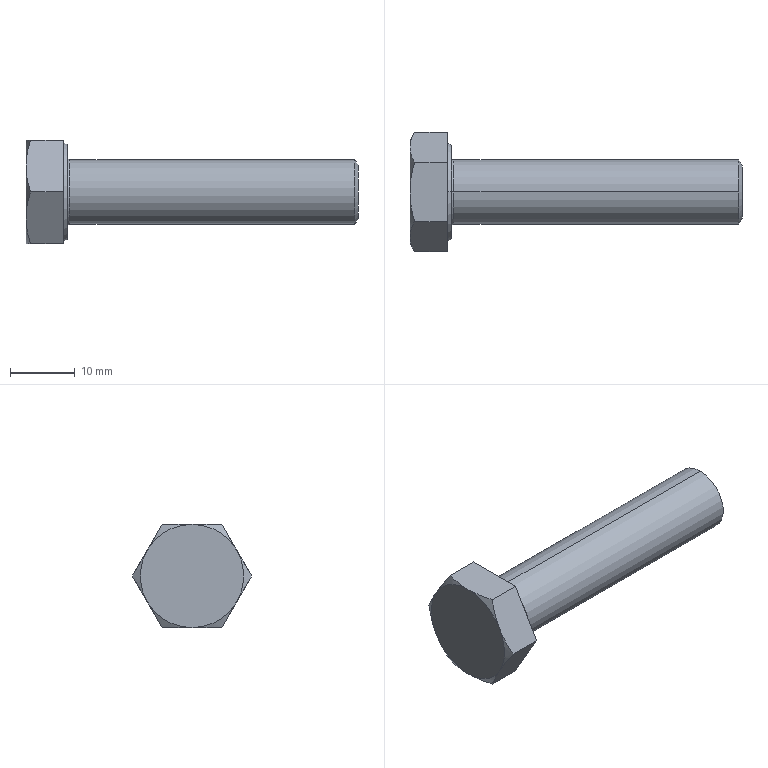Part | SolidWorks | features RevCut 3, Extrusion 1, Fillet 1, LPattern 1, Revolution 1 | 1 solid | 24 faces | box 51.4 x 18.475 x 16 mm | volume 4916 mm3 | cone 10 | plane 10 | torus 2 | cylinder 2 | commonest cylinder face diameters 10 x2
STEP:
#1=CARTESIAN_POINT('',(51.4,0.,4.134));
#2=VERTEX_POINT('',#1);
#3=CARTESIAN_POINT('',(51.4,0.,-4.134));
#4=VERTEX_POINT('',#3);
#5=CARTESIAN_POINT('',(51.4,0.,0.));
#6=DIRECTION('',(-1.,0.,0.));
#7=DIRECTION('',(0.,0.,1.));
#8=AXIS2_PLACEMENT_3D('',#5,#6,#7);
#9=CIRCLE('',#8,4.134);
#10=EDGE_CURVE('',#2,#4,#9,.T.);
#11=ORIENTED_EDGE('',*,*,#10,.T.);
#12=CARTESIAN_POINT('',(50.9,0.,-5.));
#13=VERTEX_POINT('',#12);
#14=CARTESIAN_POINT('',(50.9,0.,-5.));
#15=DIRECTION('',(-0.5,0.,-0.866));
#16=VECTOR('',#15,1000.);
#17=LINE('',#14,#16);
#18=EDGE_CURVE('',#4,#13,#17,.T.);
#19=ORIENTED_EDGE('',*,*,#18,.T.);
#20=CARTESIAN_POINT('',(50.9,0.,5.));
#21=VERTEX_POINT('',#20);
#22=CARTESIAN_POINT('',(50.9,0.,0.));
#23=DIRECTION('',(-1.,0.,0.));
#24=DIRECTION('',(0.,0.,1.));
#25=AXIS2_PLACEMENT_3D('',#22,#23,#24);
#26=CIRCLE('',#25,5.);
#27=EDGE_CURVE('',#21,#13,#26,.T.);
#28=ORIENTED_EDGE('',*,*,#27,.F.);
#29=CARTESIAN_POINT('',(50.9,0.,5.));
#30=DIRECTION('',(-0.5,0.,0.866));
#31=VECTOR('',#30,1000.);
#32=LINE('',#29,#31);
#33=EDGE_CURVE('',#2,#21,#32,.T.);
#34=ORIENTED_EDGE('',*,*,#33,.F.);
#35=EDGE_LOOP('',(#11,#19,#28,#34));
#36=FACE_OUTER_BOUND('',#35,.T.);
#37=CARTESIAN_POINT('',(50.9,0.,0.));
#38=DIRECTION('',(-1.,0.,0.));
#39=DIRECTION('',(0.,0.,1.));
#40=AXIS2_PLACEMENT_3D('',#37,#38,#39);
#41=CONICAL_SURFACE('',#40,5.,1.047);
#42=ADVANCED_FACE('',(#36),#41,.T.);
#43=CARTESIAN_POINT('',(6.8,0.,5.));
#44=VERTEX_POINT('',#43);
#45=CARTESIAN_POINT('',(6.8,0.,-5.));
#46=VERTEX_POINT('',#45);
#47=CARTESIAN_POINT('',(6.8,0.,0.));
#48=DIRECTION('',(1.,0.,0.));
#49=DIRECTION('',(0.,0.,-1.));
#50=AXIS2_PLACEMENT_3D('',#47,#48,#49);
#51=CIRCLE('',#50,5.);
#52=EDGE_CURVE('',#44,#46,#51,.T.);
#53=ORIENTED_EDGE('',*,*,#52,.F.);
#54=CARTESIAN_POINT('',(6.4,0.,5.4));
#55=VERTEX_POINT('',#54);
#56=CARTESIAN_POINT('',(6.8,0.,5.4));
#57=DIRECTION('',(0.,1.,0.));
#58=DIRECTION('',(-1.,0.,0.));
#59=AXIS2_PLACEMENT_3D('',#56,#57,#58);
#60=CIRCLE('',#59,0.4);
#61=EDGE_CURVE('',#44,#55,#60,.T.);
#62=ORIENTED_EDGE('',*,*,#61,.T.);
#63=CARTESIAN_POINT('',(6.4,0.,-5.4));
#64=VERTEX_POINT('',#63);
#65=CARTESIAN_POINT('',(6.4,0.,0.));
#66=DIRECTION('',(-1.,0.,0.));
#67=DIRECTION('',(0.,0.,-1.));
#68=AXIS2_PLACEMENT_3D('',#65,#66,#67);
#69=CIRCLE('',#68,5.4);
#70=EDGE_CURVE('',#64,#55,#69,.T.);
#71=ORIENTED_EDGE('',*,*,#70,.F.);
#72=CARTESIAN_POINT('',(6.8,0.,-5.4));
#73=DIRECTION('',(0.,-1.,0.));
#74=DIRECTION('',(1.,0.,0.));
#75=AXIS2_PLACEMENT_3D('',#72,#73,#74);
#76=CIRCLE('',#75,0.4);
#77=EDGE_CURVE('',#46,#64,#76,.T.);
#78=ORIENTED_EDGE('',*,*,#77,.F.);
#79=EDGE_LOOP('',(#53,#62,#71,#78));
#80=FACE_OUTER_BOUND('',#79,.T.);
#81=CARTESIAN_POINT('',(6.8,0.,0.));
#82=DIRECTION('',(1.,0.,0.));
#83=DIRECTION('',(0.,0.,-1.));
#84=AXIS2_PLACEMENT_3D('',#81,#82,#83);
#85=TOROIDAL_SURFACE('',#84,5.4,0.4);
#86=ADVANCED_FACE('',(#80),#85,.F.);
#87=CARTESIAN_POINT('',(6.4,0.,7.315));
#88=VERTEX_POINT('',#87);
#89=CARTESIAN_POINT('',(6.4,0.,-7.315));
#90=VERTEX_POINT('',#89);
#91=CARTESIAN_POINT('',(6.4,0.,0.));
#92=DIRECTION('',(-1.,0.,0.));
#93=DIRECTION('',(0.,0.,1.));
#94=AXIS2_PLACEMENT_3D('',#91,#92,#93);
#95=CIRCLE('',#94,7.315);
#96=EDGE_CURVE('',#88,#90,#95,.T.);
#97=ORIENTED_EDGE('',*,*,#96,.T.);
#98=CARTESIAN_POINT('',(5.8,0.,-7.661));
#99=VERTEX_POINT('',#98);
#100=CARTESIAN_POINT('',(5.8,0.,-7.661));
#101=DIRECTION('',(-0.866,0.,-0.5));
#102=VECTOR('',#101,1000.);
#103=LINE('',#100,#102);
#104=EDGE_CURVE('',#90,#99,#103,.T.);
#105=ORIENTED_EDGE('',*,*,#104,.T.);
#106=CARTESIAN_POINT('',(5.8,0.,7.661));
#107=VERTEX_POINT('',#106);
#108=CARTESIAN_POINT('',(5.8,0.,0.));
#109=DIRECTION('',(-1.,0.,0.));
#110=DIRECTION('',(0.,0.,1.));
#111=AXIS2_PLACEMENT_3D('',#108,#109,#110);
#112=CIRCLE('',#111,7.661);
#113=EDGE_CURVE('',#107,#99,#112,.T.);
#114=ORIENTED_EDGE('',*,*,#113,.F.);
#115=CARTESIAN_POINT('',(5.8,0.,7.661));
#116=DIRECTION('',(-0.866,0.,0.5));
#117=VECTOR('',#116,1000.);
#118=LINE('',#115,#117);
#119=EDGE_CURVE('',#88,#107,#118,.T.);
#120=ORIENTED_EDGE('',*,*,#119,.F.);
#121=EDGE_LOOP('',(#97,#105,#114,#120));
#122=FACE_OUTER_BOUND('',#121,.T.);
#123=CARTESIAN_POINT('',(5.8,0.,0.));
#124=DIRECTION('',(-1.,0.,0.));
#125=DIRECTION('',(0.,0.,1.));
#126=AXIS2_PLACEMENT_3D('',#123,#124,#125);
#127=CONICAL_SURFACE('',#126,7.661,0.5236);
#128=ADVANCED_FACE('',(#122),#127,.T.);
#129=ORIENTED_EDGE('',*,*,#27,.T.);
#130=CARTESIAN_POINT('',(0.,0.,-5.));
#131=DIRECTION('',(-1.,0.,0.));
#132=VECTOR('',#131,1000.);
#133=LINE('',#130,#132);
#134=EDGE_CURVE('',#13,#46,#133,.T.);
#135=ORIENTED_EDGE('',*,*,#134,.T.);
#136=CARTESIAN_POINT('',(6.8,0.,0.));
#137=DIRECTION('',(1.,0.,0.));
#138=DIRECTION('',(0.,0.,-1.));
#139=AXIS2_PLACEMENT_3D('',#136,#137,#138);
#140=CIRCLE('',#139,5.);
#141=EDGE_CURVE('',#46,#44,#140,.T.);
#142=ORIENTED_EDGE('',*,*,#141,.T.);
#143=CARTESIAN_POINT('',(0.,0.,5.));
#144=DIRECTION('',(-1.,0.,0.));
#145=VECTOR('',#144,1000.);
#146=LINE('',#143,#145);
#147=EDGE_CURVE('',#21,#44,#146,.T.);
#148=ORIENTED_EDGE('',*,*,#147,.F.);
#149=EDGE_LOOP('',(#129,#135,#142,#148));
#150=FACE_OUTER_BOUND('',#149,.T.);
#151=CARTESIAN_POINT('',(0.,0.,0.));
#152=DIRECTION('',(-1.,0.,0.));
#153=DIRECTION('',(0.,0.,1.));
#154=AXIS2_PLACEMENT_3D('',#151,#152,#153);
#155=CYLINDRICAL_SURFACE('',#154,5.);
#156=ADVANCED_FACE('',(#150),#155,.T.);
#157=ORIENTED_EDGE('',*,*,#134,.F.);
#158=CARTESIAN_POINT('',(50.9,0.,0.));
#159=DIRECTION('',(-1.,0.,0.));
#160=DIRECTION('',(0.,0.,1.));
#161=AXIS2_PLACEMENT_3D('',#158,#159,#160);
#162=CIRCLE('',#161,5.);
#163=EDGE_CURVE('',#13,#21,#162,.T.);
#164=ORIENTED_EDGE('',*,*,#163,.T.);
#165=ORIENTED_EDGE('',*,*,#147,.T.);
#166=ORIENTED_EDGE('',*,*,#52,.T.);
#167=EDGE_LOOP('',(#157,#164,#165,#166));
#168=FACE_OUTER_BOUND('',#167,.T.);
#169=CARTESIAN_POINT('',(0.,0.,0.));
#170=DIRECTION('',(-1.,0.,0.));
#171=DIRECTION('',(0.,0.,1.));
#172=AXIS2_PLACEMENT_3D('',#169,#170,#171);
#173=CYLINDRICAL_SURFACE('',#172,5.);
#174=ADVANCED_FACE('',(#168),#173,.T.);
#175=CARTESIAN_POINT('',(5.8,4.619,-8.));
#176=VERTEX_POINT('',#175);
#177=CARTESIAN_POINT('',(5.8,9.238,0.));
#178=VERTEX_POINT('',#177);
#179=CARTESIAN_POINT('',(5.8,4.619,-8.));
#180=DIRECTION('',(0.,0.5,0.866));
#181=VECTOR('',#180,1000.);
#182=LINE('',#179,#181);
#183=EDGE_CURVE('',#176,#178,#182,.T.);
#184=ORIENTED_EDGE('',*,*,#183,.F.);
#185=CARTESIAN_POINT('',(0.7145,4.619,-8.));
#186=VERTEX_POINT('',#185);
#187=CARTESIAN_POINT('',(6.4,4.619,-8.));
#188=DIRECTION('',(-1.,0.,0.));
#189=VECTOR('',#188,1000.);
#190=LINE('',#187,#189);
#191=EDGE_CURVE('',#176,#186,#190,.T.);
#192=ORIENTED_EDGE('',*,*,#191,.T.);
#193=CARTESIAN_POINT('',(0.,6.928,-4.));
#194=VERTEX_POINT('',#193);
#195=CARTESIAN_POINT('',(0.,6.928,-4.));
#196=CARTESIAN_POINT('',(0.,6.732,-4.339));
#197=CARTESIAN_POINT('',(0.01689,6.535,-4.68));
#198=CARTESIAN_POINT('',(0.08225,6.146,-5.355));
#199=CARTESIAN_POINT('',(0.1307,5.952,-5.69));
#200=CARTESIAN_POINT('',(0.3174,5.376,-6.689));
#201=CARTESIAN_POINT('',(0.497,4.996,-7.347));
#202=CARTESIAN_POINT('',(0.7145,4.619,-8.));
#203=B_SPLINE_CURVE_WITH_KNOTS('',3,(#195,#196,#197,#198,#199,#200,#201,#202),.UNSPECIFIED.,.F.,.F.,(4,2,2,4),(0.004674,0.005838,0.007002,0.00933),.UNSPECIFIED.);
#204=EDGE_CURVE('',#194,#186,#203,.T.);
#205=ORIENTED_EDGE('',*,*,#204,.F.);
#206=CARTESIAN_POINT('',(0.7145,9.238,0.));
#207=VERTEX_POINT('',#206);
#208=CARTESIAN_POINT('',(0.7145,9.238,0.));
#209=CARTESIAN_POINT('',(0.4964,8.86,-0.6543));
#210=CARTESIAN_POINT('',(0.3167,8.479,-1.313));
#211=CARTESIAN_POINT('',(0.0681,7.71,-2.646));
#212=CARTESIAN_POINT('',(0.,7.322,-3.319));
#213=CARTESIAN_POINT('',(0.,6.928,-4.));
#214=B_SPLINE_CURVE_WITH_KNOTS('',3,(#208,#209,#210,#211,#212,#213),.UNSPECIFIED.,.F.,.F.,(4,2,4),(0.000000238,0.002337,0.004674),.UNSPECIFIED.);
#215=EDGE_CURVE('',#207,#194,#214,.T.);
#216=ORIENTED_EDGE('',*,*,#215,.F.);
#217=CARTESIAN_POINT('',(6.4,9.238,0.));
#218=DIRECTION('',(-1.,0.,0.));
#219=VECTOR('',#218,1000.);
#220=LINE('',#217,#219);
#221=EDGE_CURVE('',#178,#207,#220,.T.);
#222=ORIENTED_EDGE('',*,*,#221,.F.);
#223=EDGE_LOOP('',(#184,#192,#205,#216,#222));
#224=FACE_OUTER_BOUND('',#223,.T.);
#225=CARTESIAN_POINT('',(6.4,4.619,-8.));
#226=DIRECTION('',(0.,-0.866,0.5));
#227=DIRECTION('',(0.,-0.5,-0.866));
#228=AXIS2_PLACEMENT_3D('',#225,#226,#227);
#229=PLANE('',#228);
#230=ADVANCED_FACE('',(#224),#229,.F.);
#231=CARTESIAN_POINT('',(5.8,4.619,8.));
#232=VERTEX_POINT('',#231);
#233=CARTESIAN_POINT('',(5.8,9.238,0.));
#234=DIRECTION('',(0.,-0.5,0.866));
#235=VECTOR('',#234,1000.);
#236=LINE('',#233,#235);
#237=EDGE_CURVE('',#178,#232,#236,.T.);
#238=ORIENTED_EDGE('',*,*,#237,.F.);
#239=ORIENTED_EDGE('',*,*,#221,.T.);
#240=CARTESIAN_POINT('',(0.,6.928,4.));
#241=VERTEX_POINT('',#240);
#242=CARTESIAN_POINT('',(0.,6.928,4.));
#243=CARTESIAN_POINT('',(0.,7.124,3.661));
#244=CARTESIAN_POINT('',(0.01689,7.321,3.32));
#245=CARTESIAN_POINT('',(0.08225,7.711,2.645));
#246=CARTESIAN_POINT('',(0.1307,7.904,2.31));
#247=CARTESIAN_POINT('',(0.3174,8.481,1.311));
#248=CARTESIAN_POINT('',(0.497,8.861,0.6527));
#249=CARTESIAN_POINT('',(0.7145,9.238,0.));
#250=B_SPLINE_CURVE_WITH_KNOTS('',3,(#242,#243,#244,#245,#246,#247,#248,#249),.UNSPECIFIED.,.F.,.F.,(4,2,2,4),(0.004674,0.005838,0.007002,0.00933),.UNSPECIFIED.);
#251=EDGE_CURVE('',#241,#207,#250,.T.);
#252=ORIENTED_EDGE('',*,*,#251,.F.);
#253=CARTESIAN_POINT('',(0.7145,4.619,8.));
#254=VERTEX_POINT('',#253);
#255=CARTESIAN_POINT('',(0.7145,4.619,8.));
#256=CARTESIAN_POINT('',(0.4964,4.997,7.346));
#257=CARTESIAN_POINT('',(0.3167,5.377,6.687));
#258=CARTESIAN_POINT('',(0.0681,6.146,5.354));
#259=CARTESIAN_POINT('',(0.,6.535,4.681));
#260=CARTESIAN_POINT('',(0.,6.928,4.));
#261=B_SPLINE_CURVE_WITH_KNOTS('',3,(#255,#256,#257,#258,#259,#260),.UNSPECIFIED.,.F.,.F.,(4,2,4),(0.000000238,0.002337,0.004674),.UNSPECIFIED.);
#262=EDGE_CURVE('',#254,#241,#261,.T.);
#263=ORIENTED_EDGE('',*,*,#262,.F.);
#264=CARTESIAN_POINT('',(6.4,4.619,8.));
#265=DIRECTION('',(-1.,0.,0.));
#266=VECTOR('',#265,1000.);
#267=LINE('',#264,#266);
#268=EDGE_CURVE('',#232,#254,#267,.T.);
#269=ORIENTED_EDGE('',*,*,#268,.F.);
#270=EDGE_LOOP('',(#238,#239,#252,#263,#269));
#271=FACE_OUTER_BOUND('',#270,.T.);
#272=CARTESIAN_POINT('',(6.4,9.238,0.));
#273=DIRECTION('',(0.,-0.866,-0.5));
#274=DIRECTION('',(0.,0.5,-0.866));
#275=AXIS2_PLACEMENT_3D('',#272,#273,#274);
#276=PLANE('',#275);
#277=ADVANCED_FACE('',(#271),#276,.F.);
#278=CARTESIAN_POINT('',(5.8,-4.619,8.));
#279=VERTEX_POINT('',#278);
#280=CARTESIAN_POINT('',(5.8,4.619,8.));
#281=DIRECTION('',(0.,-1.,0.));
#282=VECTOR('',#281,1000.);
#283=LINE('',#280,#282);
#284=EDGE_CURVE('',#232,#279,#283,.T.);
#285=ORIENTED_EDGE('',*,*,#284,.F.);
#286=ORIENTED_EDGE('',*,*,#268,.T.);
#287=CARTESIAN_POINT('',(0.,0.,8.));
#288=VERTEX_POINT('',#287);
#289=CARTESIAN_POINT('',(0.,0.,8.));
#290=CARTESIAN_POINT('',(0.,0.3913,8.));
#291=CARTESIAN_POINT('',(0.01678,0.7854,8.));
#292=CARTESIAN_POINT('',(0.08286,1.571,8.));
#293=CARTESIAN_POINT('',(0.1318,1.96,8.));
#294=CARTESIAN_POINT('',(0.3194,3.115,8.));
#295=CARTESIAN_POINT('',(0.4988,3.872,8.));
#296=CARTESIAN_POINT('',(0.7145,4.619,8.));
#297=B_SPLINE_CURVE_WITH_KNOTS('',3,(#289,#290,#291,#292,#293,#294,#295,#296),.UNSPECIFIED.,.F.,.F.,(4,2,2,4),(0.01337,0.01454,0.01571,0.01805),.UNSPECIFIED.);
#298=EDGE_CURVE('',#288,#254,#297,.T.);
#299=ORIENTED_EDGE('',*,*,#298,.F.);
#300=CARTESIAN_POINT('',(0.7145,-4.619,8.));
#301=VERTEX_POINT('',#300);
#302=CARTESIAN_POINT('',(0.7145,-4.619,8.));
#303=CARTESIAN_POINT('',(0.4973,-3.866,8.));
#304=CARTESIAN_POINT('',(0.3158,-3.098,8.));
#305=CARTESIAN_POINT('',(0.0673,-1.557,8.));
#306=CARTESIAN_POINT('',(0.,-0.7819,8.));
#307=CARTESIAN_POINT('',(0.,0.,8.));
#308=B_SPLINE_CURVE_WITH_KNOTS('',3,(#302,#303,#304,#305,#306,#307),.UNSPECIFIED.,.F.,.F.,(4,2,4),(0.00869,0.01103,0.01337),.UNSPECIFIED.);
#309=EDGE_CURVE('',#301,#288,#308,.T.);
#310=ORIENTED_EDGE('',*,*,#309,.F.);
#311=CARTESIAN_POINT('',(6.4,-4.619,8.));
#312=DIRECTION('',(-1.,0.,0.));
#313=VECTOR('',#312,1000.);
#314=LINE('',#311,#313);
#315=EDGE_CURVE('',#279,#301,#314,.T.);
#316=ORIENTED_EDGE('',*,*,#315,.F.);
#317=EDGE_LOOP('',(#285,#286,#299,#310,#316));
#318=FACE_OUTER_BOUND('',#317,.T.);
#319=CARTESIAN_POINT('',(6.4,4.619,8.));
#320=DIRECTION('',(0.,0.,-1.));
#321=DIRECTION('',(-1.,0.,0.));
#322=AXIS2_PLACEMENT_3D('',#319,#320,#321);
#323=PLANE('',#322);
#324=ADVANCED_FACE('',(#318),#323,.F.);
#325=CARTESIAN_POINT('',(5.8,-9.238,0.));
#326=VERTEX_POINT('',#325);
#327=CARTESIAN_POINT('',(5.8,-9.238,0.));
#328=DIRECTION('',(0.,-0.5,-0.866));
#329=VECTOR('',#328,1000.);
#330=LINE('',#327,#329);
#331=EDGE_CURVE('',#279,#326,#330,.T.);
#332=ORIENTED_EDGE('',*,*,#331,.F.);
#333=ORIENTED_EDGE('',*,*,#315,.T.);
#334=CARTESIAN_POINT('',(0.,-6.928,4.));
#335=VERTEX_POINT('',#334);
#336=CARTESIAN_POINT('',(0.,-6.928,4.));
#337=CARTESIAN_POINT('',(0.,-6.732,4.339));
#338=CARTESIAN_POINT('',(0.01689,-6.535,4.68));
#339=CARTESIAN_POINT('',(0.08225,-6.146,5.355));
#340=CARTESIAN_POINT('',(0.1307,-5.952,5.69));
#341=CARTESIAN_POINT('',(0.3174,-5.376,6.689));
#342=CARTESIAN_POINT('',(0.497,-4.996,7.347));
#343=CARTESIAN_POINT('',(0.7145,-4.619,8.));
#344=B_SPLINE_CURVE_WITH_KNOTS('',3,(#336,#337,#338,#339,#340,#341,#342,#343),.UNSPECIFIED.,.F.,.F.,(4,2,2,4),(0.004674,0.005838,0.007002,0.00933),.UNSPECIFIED.);
#345=EDGE_CURVE('',#335,#301,#344,.T.);
#346=ORIENTED_EDGE('',*,*,#345,.F.);
#347=CARTESIAN_POINT('',(0.7145,-9.238,0.));
#348=VERTEX_POINT('',#347);
#349=CARTESIAN_POINT('',(0.7145,-9.238,0.));
#350=CARTESIAN_POINT('',(0.4964,-8.86,0.6543));
#351=CARTESIAN_POINT('',(0.3167,-8.479,1.313));
#352=CARTESIAN_POINT('',(0.0681,-7.71,2.646));
#353=CARTESIAN_POINT('',(0.,-7.322,3.319));
#354=CARTESIAN_POINT('',(0.,-6.928,4.));
#355=B_SPLINE_CURVE_WITH_KNOTS('',3,(#349,#350,#351,#352,#353,#354),.UNSPECIFIED.,.F.,.F.,(4,2,4),(0.000000238,0.002337,0.004674),.UNSPECIFIED.);
#356=EDGE_CURVE('',#348,#335,#355,.T.);
#357=ORIENTED_EDGE('',*,*,#356,.F.);
#358=CARTESIAN_POINT('',(6.4,-9.238,0.));
#359=DIRECTION('',(-1.,0.,0.));
#360=VECTOR('',#359,1000.);
#361=LINE('',#358,#360);
#362=EDGE_CURVE('',#326,#348,#361,.T.);
#363=ORIENTED_EDGE('',*,*,#362,.F.);
#364=EDGE_LOOP('',(#332,#333,#346,#357,#363));
#365=FACE_OUTER_BOUND('',#364,.T.);
#366=CARTESIAN_POINT('',(6.4,-9.238,0.));
#367=DIRECTION('',(0.,0.866,-0.5));
#368=DIRECTION('',(0.,0.5,0.866));
#369=AXIS2_PLACEMENT_3D('',#366,#367,#368);
#370=PLANE('',#369);
#371=ADVANCED_FACE('',(#365),#370,.F.);
#372=CARTESIAN_POINT('',(5.8,-4.619,-8.));
#373=VERTEX_POINT('',#372);
#374=CARTESIAN_POINT('',(5.8,-4.619,-8.));
#375=DIRECTION('',(0.,0.5,-0.866));
#376=VECTOR('',#375,1000.);
#377=LINE('',#374,#376);
#378=EDGE_CURVE('',#326,#373,#377,.T.);
#379=ORIENTED_EDGE('',*,*,#378,.F.);
#380=ORIENTED_EDGE('',*,*,#362,.T.);
#381=CARTESIAN_POINT('',(0.,-6.928,-4.));
#382=VERTEX_POINT('',#381);
#383=CARTESIAN_POINT('',(0.,-6.928,-4.));
#384=CARTESIAN_POINT('',(0.,-7.124,-3.661));
#385=CARTESIAN_POINT('',(0.01689,-7.321,-3.32));
#386=CARTESIAN_POINT('',(0.08225,-7.711,-2.645));
#387=CARTESIAN_POINT('',(0.1307,-7.904,-2.31));
#388=CARTESIAN_POINT('',(0.3174,-8.481,-1.311));
#389=CARTESIAN_POINT('',(0.497,-8.861,-0.6527));
#390=CARTESIAN_POINT('',(0.7145,-9.238,0.));
#391=B_SPLINE_CURVE_WITH_KNOTS('',3,(#383,#384,#385,#386,#387,#388,#389,#390),.UNSPECIFIED.,.F.,.F.,(4,2,2,4),(0.004674,0.005838,0.007002,0.00933),.UNSPECIFIED.);
#392=EDGE_CURVE('',#382,#348,#391,.T.);
#393=ORIENTED_EDGE('',*,*,#392,.F.);
#394=CARTESIAN_POINT('',(0.7145,-4.619,-8.));
#395=VERTEX_POINT('',#394);
#396=CARTESIAN_POINT('',(0.7145,-4.619,-8.));
#397=CARTESIAN_POINT('',(0.4964,-4.997,-7.346));
#398=CARTESIAN_POINT('',(0.3167,-5.377,-6.687));
#399=CARTESIAN_POINT('',(0.0681,-6.146,-5.354));
#400=CARTESIAN_POINT('',(0.,-6.535,-4.681));
#401=CARTESIAN_POINT('',(0.,-6.928,-4.));
#402=B_SPLINE_CURVE_WITH_KNOTS('',3,(#396,#397,#398,#399,#400,#401),.UNSPECIFIED.,.F.,.F.,(4,2,4),(0.000000238,0.002337,0.004674),.UNSPECIFIED.);
#403=EDGE_CURVE('',#395,#382,#402,.T.);
#404=ORIENTED_EDGE('',*,*,#403,.F.);
#405=CARTESIAN_POINT('',(6.4,-4.619,-8.));
#406=DIRECTION('',(-1.,0.,0.));
#407=VECTOR('',#406,1000.);
#408=LINE('',#405,#407);
#409=EDGE_CURVE('',#373,#395,#408,.T.);
#410=ORIENTED_EDGE('',*,*,#409,.F.);
#411=EDGE_LOOP('',(#379,#380,#393,#404,#410));
#412=FACE_OUTER_BOUND('',#411,.T.);
#413=CARTESIAN_POINT('',(6.4,-4.619,-8.));
#414=DIRECTION('',(0.,0.866,0.5));
#415=DIRECTION('',(0.,-0.5,0.866));
#416=AXIS2_PLACEMENT_3D('',#413,#414,#415);
#417=PLANE('',#416);
#418=ADVANCED_FACE('',(#412),#417,.F.);
#419=CARTESIAN_POINT('',(5.8,4.619,-8.));
#420=DIRECTION('',(0.,1.,0.));
#421=VECTOR('',#420,1000.);
#422=LINE('',#419,#421);
#423=EDGE_CURVE('',#373,#176,#422,.T.);
#424=ORIENTED_EDGE('',*,*,#423,.F.);
#425=ORIENTED_EDGE('',*,*,#409,.T.);
#426=CARTESIAN_POINT('',(0.,0.,-8.));
#427=VERTEX_POINT('',#426);
#428=CARTESIAN_POINT('',(0.,0.,-8.));
#429=CARTESIAN_POINT('',(0.,-0.7819,-8.));
#430=CARTESIAN_POINT('',(0.0673,-1.557,-8.));
#431=CARTESIAN_POINT('',(0.3158,-3.098,-8.));
#432=CARTESIAN_POINT('',(0.4973,-3.866,-8.));
#433=CARTESIAN_POINT('',(0.7145,-4.619,-8.));
#434=B_SPLINE_CURVE_WITH_KNOTS('',3,(#428,#429,#430,#431,#432,#433),.UNSPECIFIED.,.F.,.F.,(4,2,4),(0.02753,0.02987,0.03221),.UNSPECIFIED.);
#435=EDGE_CURVE('',#427,#395,#434,.T.);
#436=ORIENTED_EDGE('',*,*,#435,.F.);
#437=CARTESIAN_POINT('',(0.7145,4.619,-8.));
#438=CARTESIAN_POINT('',(0.4988,3.872,-8.));
#439=CARTESIAN_POINT('',(0.3194,3.115,-8.));
#440=CARTESIAN_POINT('',(0.1318,1.96,-8.));
#441=CARTESIAN_POINT('',(0.08286,1.571,-8.));
#442=CARTESIAN_POINT('',(0.01678,0.7854,-8.));
#443=CARTESIAN_POINT('',(0.,0.3913,-8.));
#444=CARTESIAN_POINT('',(0.,0.,-8.));
#445=B_SPLINE_CURVE_WITH_KNOTS('',3,(#437,#438,#439,#440,#441,#442,#443,#444),.UNSPECIFIED.,.F.,.F.,(4,2,2,4),(0.02285,0.02519,0.02636,0.02753),.UNSPECIFIED.);
#446=EDGE_CURVE('',#186,#427,#445,.T.);
#447=ORIENTED_EDGE('',*,*,#446,.F.);
#448=ORIENTED_EDGE('',*,*,#191,.F.);
#449=EDGE_LOOP('',(#424,#425,#436,#447,#448));
#450=FACE_OUTER_BOUND('',#449,.T.);
#451=CARTESIAN_POINT('',(6.4,4.619,-8.));
#452=DIRECTION('',(0.,0.,1.));
#453=DIRECTION('',(0.,-1.,0.));
#454=AXIS2_PLACEMENT_3D('',#451,#452,#453);
#455=PLANE('',#454);
#456=ADVANCED_FACE('',(#450),#455,.F.);
#457=ORIENTED_EDGE('',*,*,#403,.T.);
#458=CARTESIAN_POINT('',(0.,0.,0.));
#459=DIRECTION('',(1.,0.,0.));
#460=DIRECTION('',(0.,0.,-1.));
#461=AXIS2_PLACEMENT_3D('',#458,#459,#460);
#462=CIRCLE('',#461,8.);
#463=EDGE_CURVE('',#382,#427,#462,.T.);
#464=ORIENTED_EDGE('',*,*,#463,.T.);
#465=ORIENTED_EDGE('',*,*,#435,.T.);
#466=EDGE_LOOP('',(#457,#464,#465));
#467=FACE_OUTER_BOUND('',#466,.T.);
#468=CARTESIAN_POINT('',(0.,0.,0.));
#469=DIRECTION('',(1.,0.,0.));
#470=DIRECTION('',(0.,0.,-1.));
#471=AXIS2_PLACEMENT_3D('',#468,#469,#470);
#472=CONICAL_SURFACE('',#471,8.,1.047);
#473=ADVANCED_FACE('',(#467),#472,.T.);
#474=ORIENTED_EDGE('',*,*,#356,.T.);
#475=CARTESIAN_POINT('',(0.,0.,0.));
#476=DIRECTION('',(1.,0.,0.));
#477=DIRECTION('',(0.,0.,-1.));
#478=AXIS2_PLACEMENT_3D('',#475,#476,#477);
#479=CIRCLE('',#478,8.);
#480=EDGE_CURVE('',#335,#382,#479,.T.);
#481=ORIENTED_EDGE('',*,*,#480,.T.);
#482=ORIENTED_EDGE('',*,*,#392,.T.);
#483=EDGE_LOOP('',(#474,#481,#482));
#484=FACE_OUTER_BOUND('',#483,.T.);
#485=CARTESIAN_POINT('',(0.,0.,0.));
#486=DIRECTION('',(1.,0.,0.));
#487=DIRECTION('',(0.,0.,-1.));
#488=AXIS2_PLACEMENT_3D('',#485,#486,#487);
#489=CONICAL_SURFACE('',#488,8.,1.047);
#490=ADVANCED_FACE('',(#484),#489,.T.);
#491=ORIENTED_EDGE('',*,*,#309,.T.);
#492=CARTESIAN_POINT('',(0.,0.,0.));
#493=DIRECTION('',(1.,0.,0.));
#494=DIRECTION('',(0.,0.,-1.));
#495=AXIS2_PLACEMENT_3D('',#492,#493,#494);
#496=CIRCLE('',#495,8.);
#497=EDGE_CURVE('',#288,#335,#496,.T.);
#498=ORIENTED_EDGE('',*,*,#497,.T.);
#499=ORIENTED_EDGE('',*,*,#345,.T.);
#500=EDGE_LOOP('',(#491,#498,#499));
#501=FACE_OUTER_BOUND('',#500,.T.);
#502=CARTESIAN_POINT('',(0.,0.,0.));
#503=DIRECTION('',(1.,0.,0.));
#504=DIRECTION('',(0.,0.,-1.));
#505=AXIS2_PLACEMENT_3D('',#502,#503,#504);
#506=CONICAL_SURFACE('',#505,8.,1.047);
#507=ADVANCED_FACE('',(#501),#506,.T.);
#508=ORIENTED_EDGE('',*,*,#298,.T.);
#509=ORIENTED_EDGE('',*,*,#262,.T.);
#510=CARTESIAN_POINT('',(0.,0.,0.));
#511=DIRECTION('',(-1.,0.,0.));
#512=DIRECTION('',(0.,0.,1.));
#513=AXIS2_PLACEMENT_3D('',#510,#511,#512);
#514=CIRCLE('',#513,8.);
#515=EDGE_CURVE('',#288,#241,#514,.T.);
#516=ORIENTED_EDGE('',*,*,#515,.F.);
#517=EDGE_LOOP('',(#508,#509,#516));
#518=FACE_OUTER_BOUND('',#517,.T.);
#519=CARTESIAN_POINT('',(0.,0.,0.));
#520=DIRECTION('',(1.,0.,0.));
#521=DIRECTION('',(0.,0.,-1.));
#522=AXIS2_PLACEMENT_3D('',#519,#520,#521);
#523=CONICAL_SURFACE('',#522,8.,1.047);
#524=ADVANCED_FACE('',(#518),#523,.T.);
#525=ORIENTED_EDGE('',*,*,#251,.T.);
#526=ORIENTED_EDGE('',*,*,#215,.T.);
#527=CARTESIAN_POINT('',(0.,0.,0.));
#528=DIRECTION('',(1.,0.,0.));
#529=DIRECTION('',(0.,0.,-1.));
#530=AXIS2_PLACEMENT_3D('',#527,#528,#529);
#531=CIRCLE('',#530,8.);
#532=EDGE_CURVE('',#194,#241,#531,.T.);
#533=ORIENTED_EDGE('',*,*,#532,.T.);
#534=EDGE_LOOP('',(#525,#526,#533));
#535=FACE_OUTER_BOUND('',#534,.T.);
#536=CARTESIAN_POINT('',(0.,0.,0.));
#537=DIRECTION('',(1.,0.,0.));
#538=DIRECTION('',(0.,0.,-1.));
#539=AXIS2_PLACEMENT_3D('',#536,#537,#538);
#540=CONICAL_SURFACE('',#539,8.,1.047);
#541=ADVANCED_FACE('',(#535),#540,.T.);
#542=ORIENTED_EDGE('',*,*,#204,.T.);
#543=ORIENTED_EDGE('',*,*,#446,.T.);
#544=CARTESIAN_POINT('',(0.,0.,0.));
#545=DIRECTION('',(1.,0.,0.));
#546=DIRECTION('',(0.,0.,-1.));
#547=AXIS2_PLACEMENT_3D('',#544,#545,#546);
#548=CIRCLE('',#547,8.);
#549=EDGE_CURVE('',#427,#194,#548,.T.);
#550=ORIENTED_EDGE('',*,*,#549,.T.);
#551=EDGE_LOOP('',(#542,#543,#550));
#552=FACE_OUTER_BOUND('',#551,.T.);
#553=CARTESIAN_POINT('',(0.,0.,0.));
#554=DIRECTION('',(1.,0.,0.));
#555=DIRECTION('',(0.,0.,-1.));
#556=AXIS2_PLACEMENT_3D('',#553,#554,#555);
#557=CONICAL_SURFACE('',#556,8.,1.047);
#558=ADVANCED_FACE('',(#552),#557,.T.);
#559=ORIENTED_EDGE('',*,*,#549,.F.);
#560=ORIENTED_EDGE('',*,*,#463,.F.);
#561=ORIENTED_EDGE('',*,*,#480,.F.);
#562=ORIENTED_EDGE('',*,*,#497,.F.);
#563=ORIENTED_EDGE('',*,*,#515,.T.);
#564=ORIENTED_EDGE('',*,*,#532,.F.);
#565=EDGE_LOOP('',(#559,#560,#561,#562,#563,#564));
#566=FACE_OUTER_BOUND('',#565,.T.);
#567=CARTESIAN_POINT('',(0.,9.238,0.));
#568=DIRECTION('',(1.,0.,0.));
#569=DIRECTION('',(0.,0.,-1.));
#570=AXIS2_PLACEMENT_3D('',#567,#568,#569);
#571=PLANE('',#570);
#572=ADVANCED_FACE('',(#566),#571,.F.);
#573=ORIENTED_EDGE('',*,*,#113,.T.);
#574=CARTESIAN_POINT('',(5.8,0.,0.));
#575=DIRECTION('',(-1.,0.,0.));
#576=DIRECTION('',(0.,0.,1.));
#577=AXIS2_PLACEMENT_3D('',#574,#575,#576);
#578=CIRCLE('',#577,7.661);
#579=EDGE_CURVE('',#99,#107,#578,.T.);
#580=ORIENTED_EDGE('',*,*,#579,.T.);
#581=EDGE_LOOP('',(#573,#580));
#582=FACE_BOUND('',#581,.T.);
#583=ORIENTED_EDGE('',*,*,#183,.T.);
#584=ORIENTED_EDGE('',*,*,#237,.T.);
#585=ORIENTED_EDGE('',*,*,#284,.T.);
#586=ORIENTED_EDGE('',*,*,#331,.T.);
#587=ORIENTED_EDGE('',*,*,#378,.T.);
#588=ORIENTED_EDGE('',*,*,#423,.T.);
#589=EDGE_LOOP('',(#583,#584,#585,#586,#587,#588));
#590=FACE_OUTER_BOUND('',#589,.T.);
#591=CARTESIAN_POINT('',(5.8,7.661,0.));
#592=DIRECTION('',(1.,0.,0.));
#593=DIRECTION('',(0.,0.,-1.));
#594=AXIS2_PLACEMENT_3D('',#591,#592,#593);
#595=PLANE('',#594);
#596=ADVANCED_FACE('',(#582,#590),#595,.T.);
#597=ORIENTED_EDGE('',*,*,#104,.F.);
#598=CARTESIAN_POINT('',(6.4,0.,0.));
#599=DIRECTION('',(-1.,0.,0.));
#600=DIRECTION('',(0.,0.,1.));
#601=AXIS2_PLACEMENT_3D('',#598,#599,#600);
#602=CIRCLE('',#601,7.315);
#603=EDGE_CURVE('',#90,#88,#602,.T.);
#604=ORIENTED_EDGE('',*,*,#603,.T.);
#605=ORIENTED_EDGE('',*,*,#119,.T.);
#606=ORIENTED_EDGE('',*,*,#579,.F.);
#607=EDGE_LOOP('',(#597,#604,#605,#606));
#608=FACE_OUTER_BOUND('',#607,.T.);
#609=CARTESIAN_POINT('',(5.8,0.,0.));
#610=DIRECTION('',(-1.,0.,0.));
#611=DIRECTION('',(0.,0.,1.));
#612=AXIS2_PLACEMENT_3D('',#609,#610,#611);
#613=CONICAL_SURFACE('',#612,7.661,0.5236);
#614=ADVANCED_FACE('',(#608),#613,.T.);
#615=ORIENTED_EDGE('',*,*,#70,.T.);
#616=CARTESIAN_POINT('',(6.4,0.,0.));
#617=DIRECTION('',(-1.,0.,0.));
#618=DIRECTION('',(0.,0.,-1.));
#619=AXIS2_PLACEMENT_3D('',#616,#617,#618);
#620=CIRCLE('',#619,5.4);
#621=EDGE_CURVE('',#55,#64,#620,.T.);
#622=ORIENTED_EDGE('',*,*,#621,.T.);
#623=EDGE_LOOP('',(#615,#622));
#624=FACE_BOUND('',#623,.T.);
#625=ORIENTED_EDGE('',*,*,#96,.F.);
#626=ORIENTED_EDGE('',*,*,#603,.F.);
#627=EDGE_LOOP('',(#625,#626));
#628=FACE_OUTER_BOUND('',#627,.T.);
#629=CARTESIAN_POINT('',(6.4,9.238,0.));
#630=DIRECTION('',(1.,0.,0.));
#631=DIRECTION('',(0.,0.,-1.));
#632=AXIS2_PLACEMENT_3D('',#629,#630,#631);
#633=PLANE('',#632);
#634=ADVANCED_FACE('',(#624,#628),#633,.T.);
#635=ORIENTED_EDGE('',*,*,#61,.F.);
#636=ORIENTED_EDGE('',*,*,#141,.F.);
#637=ORIENTED_EDGE('',*,*,#77,.T.);
#638=ORIENTED_EDGE('',*,*,#621,.F.);
#639=EDGE_LOOP('',(#635,#636,#637,#638));
#640=FACE_OUTER_BOUND('',#639,.T.);
#641=CARTESIAN_POINT('',(6.8,0.,0.));
#642=DIRECTION('',(1.,0.,0.));
#643=DIRECTION('',(0.,0.,-1.));
#644=AXIS2_PLACEMENT_3D('',#641,#642,#643);
#645=TOROIDAL_SURFACE('',#644,5.4,0.4);
#646=ADVANCED_FACE('',(#640),#645,.F.);
#647=ORIENTED_EDGE('',*,*,#18,.F.);
#648=CARTESIAN_POINT('',(51.4,0.,0.));
#649=DIRECTION('',(-1.,0.,0.));
#650=DIRECTION('',(0.,0.,1.));
#651=AXIS2_PLACEMENT_3D('',#648,#649,#650);
#652=CIRCLE('',#651,4.134);
#653=EDGE_CURVE('',#4,#2,#652,.T.);
#654=ORIENTED_EDGE('',*,*,#653,.T.);
#655=ORIENTED_EDGE('',*,*,#33,.T.);
#656=ORIENTED_EDGE('',*,*,#163,.F.);
#657=EDGE_LOOP('',(#647,#654,#655,#656));
#658=FACE_OUTER_BOUND('',#657,.T.);
#659=CARTESIAN_POINT('',(50.9,0.,0.));
#660=DIRECTION('',(-1.,0.,0.));
#661=DIRECTION('',(0.,0.,1.));
#662=AXIS2_PLACEMENT_3D('',#659,#660,#661);
#663=CONICAL_SURFACE('',#662,5.,1.047);
#664=ADVANCED_FACE('',(#658),#663,.T.);
#665=ORIENTED_EDGE('',*,*,#10,.F.);
#666=ORIENTED_EDGE('',*,*,#653,.F.);
#667=EDGE_LOOP('',(#665,#666));
#668=FACE_OUTER_BOUND('',#667,.T.);
#669=CARTESIAN_POINT('',(51.4,0.,0.));
#670=DIRECTION('',(-1.,0.,0.));
#671=DIRECTION('',(0.,0.,1.));
#672=AXIS2_PLACEMENT_3D('',#669,#670,#671);
#673=PLANE('',#672);
#674=ADVANCED_FACE('',(#668),#673,.F.);
#675=CLOSED_SHELL('',(#42,#86,#128,#156,#174,#230,#277,#324,#371,#418,#456,#473,#490,#507,#524,#541,#558,#572,#596,#614,#634,#646,#664,#674));
#676=MANIFOLD_SOLID_BREP('',#675);
#677=CARTESIAN_POINT('',(0.,0.,0.));
#678=DIRECTION('',(0.,0.,1.));
#679=DIRECTION('',(1.,0.,0.));
#680=AXIS2_PLACEMENT_3D('',#677,#678,#679);
#681=(LENGTH_UNIT()NAMED_UNIT(*)SI_UNIT(.MILLI.,.METRE.));
#682=UNCERTAINTY_MEASURE_WITH_UNIT(LENGTH_MEASURE(0.00001),#681,'','');
#683=(NAMED_UNIT(*)PLANE_ANGLE_UNIT()SI_UNIT($,.RADIAN.));
#684=(NAMED_UNIT(*)SI_UNIT($,.STERADIAN.)SOLID_ANGLE_UNIT());
#685=(GEOMETRIC_REPRESENTATION_CONTEXT(3)GLOBAL_UNCERTAINTY_ASSIGNED_CONTEXT((#682))GLOBAL_UNIT_ASSIGNED_CONTEXT((#681,#683,#684))REPRESENTATION_CONTEXT('',''));
#686=ADVANCED_BREP_SHAPE_REPRESENTATION('',(#676,#680),#685);